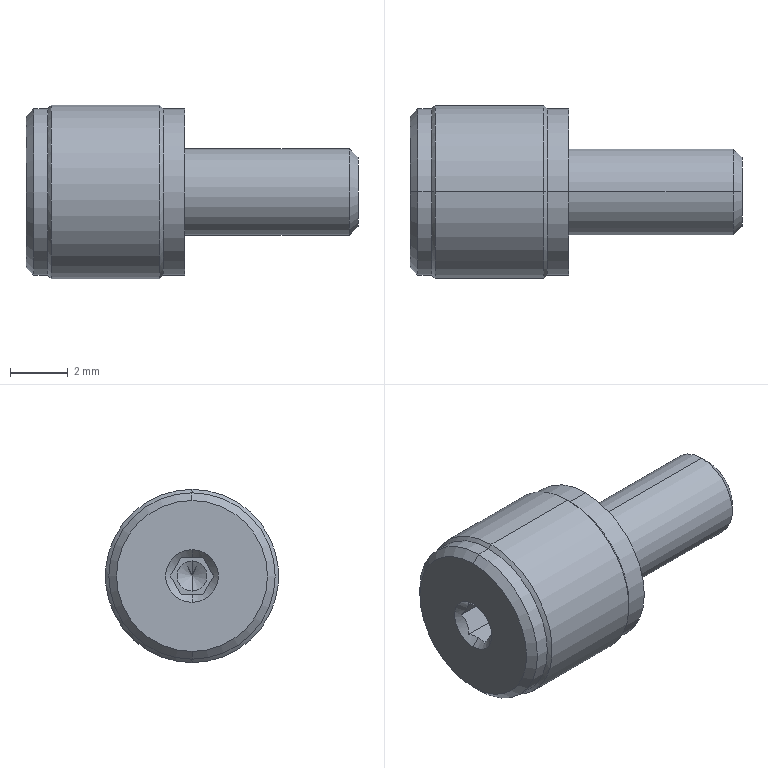Part | SolidWorks | features ICE 1, RevCut 1, Revolution 1 | 1 solid | 32 faces | box 11.5 x 6 x 6 mm | volume 189.881 mm3 | cone 12 | cylinder 10 | plane 10 | commonest cylinder face diameters 5.76 x4 1.04 x2 3 x2 6 x2
STEP:
#1=CARTESIAN_POINT('',(-3.05,0.,-0.52));
#2=VERTEX_POINT('',#1);
#3=CARTESIAN_POINT('',(-3.05,0.,0.52));
#4=VERTEX_POINT('',#3);
#5=CARTESIAN_POINT('',(-3.05,0.,0.));
#6=DIRECTION('',(-1.,0.,0.));
#7=DIRECTION('',(0.,0.,1.));
#8=AXIS2_PLACEMENT_3D('',#5,#6,#7);
#9=CIRCLE('',#8,0.52);
#10=EDGE_CURVE('',#2,#4,#9,.T.);
#11=ORIENTED_EDGE('',*,*,#10,.F.);
#12=CARTESIAN_POINT('',(-3.667,0.,-0.52));
#13=VERTEX_POINT('',#12);
#14=CARTESIAN_POINT('',(-2.75,0.,-0.52));
#15=DIRECTION('',(-1.,0.,0.));
#16=VECTOR('',#15,1000.);
#17=LINE('',#14,#16);
#18=EDGE_CURVE('',#2,#13,#17,.T.);
#19=ORIENTED_EDGE('',*,*,#18,.T.);
#20=CARTESIAN_POINT('',(-3.667,0.,0.52));
#21=VERTEX_POINT('',#20);
#22=CARTESIAN_POINT('',(-3.667,0.,0.));
#23=DIRECTION('',(1.,0.,0.));
#24=DIRECTION('',(0.,0.,-1.));
#25=AXIS2_PLACEMENT_3D('',#22,#23,#24);
#26=CIRCLE('',#25,0.52);
#27=EDGE_CURVE('',#21,#13,#26,.T.);
#28=ORIENTED_EDGE('',*,*,#27,.F.);
#29=CARTESIAN_POINT('',(-2.75,0.,0.52));
#30=DIRECTION('',(-1.,0.,0.));
#31=VECTOR('',#30,1000.);
#32=LINE('',#29,#31);
#33=EDGE_CURVE('',#4,#21,#32,.T.);
#34=ORIENTED_EDGE('',*,*,#33,.F.);
#35=EDGE_LOOP('',(#11,#19,#28,#34));
#36=FACE_OUTER_BOUND('',#35,.T.);
#37=CARTESIAN_POINT('',(-2.75,0.,0.));
#38=DIRECTION('',(-1.,0.,0.));
#39=DIRECTION('',(0.,0.,1.));
#40=AXIS2_PLACEMENT_3D('',#37,#38,#39);
#41=CYLINDRICAL_SURFACE('',#40,0.52);
#42=ADVANCED_FACE('',(#36),#41,.F.);
#43=CARTESIAN_POINT('',(-2.75,0.,0.));
#44=VERTEX_POINT('',#43);
#45=CARTESIAN_POINT('',(-2.75,0.,0.));
#46=DIRECTION('',(-0.5,0.,0.866));
#47=VECTOR('',#46,1000.);
#48=LINE('',#45,#47);
#49=EDGE_CURVE('',#44,#4,#48,.T.);
#50=ORIENTED_EDGE('',*,*,#49,.F.);
#51=CARTESIAN_POINT('',(-2.75,0.,0.));
#52=DIRECTION('',(-0.5,0.,-0.866));
#53=VECTOR('',#52,1000.);
#54=LINE('',#51,#53);
#55=EDGE_CURVE('',#44,#2,#54,.T.);
#56=ORIENTED_EDGE('',*,*,#55,.T.);
#57=ORIENTED_EDGE('',*,*,#10,.T.);
#58=EDGE_LOOP('',(#50,#56,#57));
#59=FACE_OUTER_BOUND('',#58,.T.);
#60=CARTESIAN_POINT('',(-1002.75,0.,0.));
#61=DIRECTION('',(-1.,0.,0.));
#62=DIRECTION('',(0.,0.,1.));
#63=AXIS2_PLACEMENT_3D('',#60,#61,#62);
#64=CONICAL_SURFACE('',#63,1732.051,1.047);
#65=ADVANCED_FACE('',(#59),#64,.F.);
#66=CARTESIAN_POINT('',(6.,0.,1.194));
#67=VERTEX_POINT('',#66);
#68=CARTESIAN_POINT('',(6.,0.,-1.194));
#69=VERTEX_POINT('',#68);
#70=CARTESIAN_POINT('',(6.,0.,0.));
#71=DIRECTION('',(-1.,0.,0.));
#72=DIRECTION('',(0.,0.,1.));
#73=AXIS2_PLACEMENT_3D('',#70,#71,#72);
#74=CIRCLE('',#73,1.194);
#75=EDGE_CURVE('',#67,#69,#74,.T.);
#76=ORIENTED_EDGE('',*,*,#75,.T.);
#77=CARTESIAN_POINT('',(5.694,0.,-1.5));
#78=VERTEX_POINT('',#77);
#79=CARTESIAN_POINT('',(6.,0.,-1.194));
#80=DIRECTION('',(-0.7071,0.,-0.7071));
#81=VECTOR('',#80,1000.);
#82=LINE('',#79,#81);
#83=EDGE_CURVE('',#69,#78,#82,.T.);
#84=ORIENTED_EDGE('',*,*,#83,.T.);
#85=CARTESIAN_POINT('',(5.694,0.,1.5));
#86=VERTEX_POINT('',#85);
#87=CARTESIAN_POINT('',(5.694,0.,0.));
#88=DIRECTION('',(-1.,0.,0.));
#89=DIRECTION('',(0.,0.,1.));
#90=AXIS2_PLACEMENT_3D('',#87,#88,#89);
#91=CIRCLE('',#90,1.5);
#92=EDGE_CURVE('',#86,#78,#91,.T.);
#93=ORIENTED_EDGE('',*,*,#92,.F.);
#94=CARTESIAN_POINT('',(6.,0.,1.194));
#95=DIRECTION('',(-0.7071,0.,0.7071));
#96=VECTOR('',#95,1000.);
#97=LINE('',#94,#96);
#98=EDGE_CURVE('',#67,#86,#97,.T.);
#99=ORIENTED_EDGE('',*,*,#98,.F.);
#100=EDGE_LOOP('',(#76,#84,#93,#99));
#101=FACE_OUTER_BOUND('',#100,.T.);
#102=CARTESIAN_POINT('',(6.,0.,0.));
#103=DIRECTION('',(-1.,0.,0.));
#104=DIRECTION('',(0.,0.,1.));
#105=AXIS2_PLACEMENT_3D('',#102,#103,#104);
#106=CONICAL_SURFACE('',#105,1.194,0.7854);
#107=ADVANCED_FACE('',(#101),#106,.T.);
#108=ORIENTED_EDGE('',*,*,#92,.T.);
#109=CARTESIAN_POINT('',(0.,0.,-1.5));
#110=VERTEX_POINT('',#109);
#111=CARTESIAN_POINT('',(6.,0.,-1.5));
#112=DIRECTION('',(-1.,0.,0.));
#113=VECTOR('',#112,1000.);
#114=LINE('',#111,#113);
#115=EDGE_CURVE('',#78,#110,#114,.T.);
#116=ORIENTED_EDGE('',*,*,#115,.T.);
#117=CARTESIAN_POINT('',(0.,0.,1.5));
#118=VERTEX_POINT('',#117);
#119=CARTESIAN_POINT('',(0.,0.,0.));
#120=DIRECTION('',(-1.,0.,0.));
#121=DIRECTION('',(0.,0.,1.));
#122=AXIS2_PLACEMENT_3D('',#119,#120,#121);
#123=CIRCLE('',#122,1.5);
#124=EDGE_CURVE('',#118,#110,#123,.T.);
#125=ORIENTED_EDGE('',*,*,#124,.F.);
#126=CARTESIAN_POINT('',(6.,0.,1.5));
#127=DIRECTION('',(-1.,0.,0.));
#128=VECTOR('',#127,1000.);
#129=LINE('',#126,#128);
#130=EDGE_CURVE('',#86,#118,#129,.T.);
#131=ORIENTED_EDGE('',*,*,#130,.F.);
#132=EDGE_LOOP('',(#108,#116,#125,#131));
#133=FACE_OUTER_BOUND('',#132,.T.);
#134=CARTESIAN_POINT('',(6.,0.,0.));
#135=DIRECTION('',(-1.,0.,0.));
#136=DIRECTION('',(0.,0.,1.));
#137=AXIS2_PLACEMENT_3D('',#134,#135,#136);
#138=CYLINDRICAL_SURFACE('',#137,1.5);
#139=ADVANCED_FACE('',(#133),#138,.T.);
#140=CARTESIAN_POINT('',(0.,0.,2.88));
#141=VERTEX_POINT('',#140);
#142=CARTESIAN_POINT('',(0.,0.,-2.88));
#143=VERTEX_POINT('',#142);
#144=CARTESIAN_POINT('',(0.,0.,0.));
#145=DIRECTION('',(-1.,0.,0.));
#146=DIRECTION('',(0.,0.,1.));
#147=AXIS2_PLACEMENT_3D('',#144,#145,#146);
#148=CIRCLE('',#147,2.88);
#149=EDGE_CURVE('',#141,#143,#148,.T.);
#150=ORIENTED_EDGE('',*,*,#149,.T.);
#151=CARTESIAN_POINT('',(-0.75,0.,-2.88));
#152=VERTEX_POINT('',#151);
#153=CARTESIAN_POINT('',(6.,0.,-2.88));
#154=DIRECTION('',(-1.,0.,0.));
#155=VECTOR('',#154,1000.);
#156=LINE('',#153,#155);
#157=EDGE_CURVE('',#143,#152,#156,.T.);
#158=ORIENTED_EDGE('',*,*,#157,.T.);
#159=CARTESIAN_POINT('',(-0.75,0.,2.88));
#160=VERTEX_POINT('',#159);
#161=CARTESIAN_POINT('',(-0.75,0.,0.));
#162=DIRECTION('',(-1.,0.,0.));
#163=DIRECTION('',(0.,0.,1.));
#164=AXIS2_PLACEMENT_3D('',#161,#162,#163);
#165=CIRCLE('',#164,2.88);
#166=EDGE_CURVE('',#160,#152,#165,.T.);
#167=ORIENTED_EDGE('',*,*,#166,.F.);
#168=CARTESIAN_POINT('',(6.,0.,2.88));
#169=DIRECTION('',(-1.,0.,0.));
#170=VECTOR('',#169,1000.);
#171=LINE('',#168,#170);
#172=EDGE_CURVE('',#141,#160,#171,.T.);
#173=ORIENTED_EDGE('',*,*,#172,.F.);
#174=EDGE_LOOP('',(#150,#158,#167,#173));
#175=FACE_OUTER_BOUND('',#174,.T.);
#176=CARTESIAN_POINT('',(6.,0.,0.));
#177=DIRECTION('',(-1.,0.,0.));
#178=DIRECTION('',(0.,0.,1.));
#179=AXIS2_PLACEMENT_3D('',#176,#177,#178);
#180=CYLINDRICAL_SURFACE('',#179,2.88);
#181=ADVANCED_FACE('',(#175),#180,.T.);
#182=ORIENTED_EDGE('',*,*,#166,.T.);
#183=CARTESIAN_POINT('',(-0.87,0.,-3.));
#184=VERTEX_POINT('',#183);
#185=CARTESIAN_POINT('',(-0.75,0.,-2.88));
#186=DIRECTION('',(-0.7071,0.,-0.7071));
#187=VECTOR('',#186,1000.);
#188=LINE('',#185,#187);
#189=EDGE_CURVE('',#152,#184,#188,.T.);
#190=ORIENTED_EDGE('',*,*,#189,.T.);
#191=CARTESIAN_POINT('',(-0.87,0.,3.));
#192=VERTEX_POINT('',#191);
#193=CARTESIAN_POINT('',(-0.87,0.,0.));
#194=DIRECTION('',(-1.,0.,0.));
#195=DIRECTION('',(0.,0.,1.));
#196=AXIS2_PLACEMENT_3D('',#193,#194,#195);
#197=CIRCLE('',#196,3.);
#198=EDGE_CURVE('',#192,#184,#197,.T.);
#199=ORIENTED_EDGE('',*,*,#198,.F.);
#200=CARTESIAN_POINT('',(-0.75,0.,2.88));
#201=DIRECTION('',(-0.7071,0.,0.7071));
#202=VECTOR('',#201,1000.);
#203=LINE('',#200,#202);
#204=EDGE_CURVE('',#160,#192,#203,.T.);
#205=ORIENTED_EDGE('',*,*,#204,.F.);
#206=EDGE_LOOP('',(#182,#190,#199,#205));
#207=FACE_OUTER_BOUND('',#206,.T.);
#208=CARTESIAN_POINT('',(-0.75,0.,0.));
#209=DIRECTION('',(-1.,0.,0.));
#210=DIRECTION('',(0.,0.,1.));
#211=AXIS2_PLACEMENT_3D('',#208,#209,#210);
#212=CONICAL_SURFACE('',#211,2.88,0.7854);
#213=ADVANCED_FACE('',(#207),#212,.T.);
#214=ORIENTED_EDGE('',*,*,#198,.T.);
#215=CARTESIAN_POINT('',(-4.63,0.,-3.));
#216=VERTEX_POINT('',#215);
#217=CARTESIAN_POINT('',(6.,0.,-3.));
#218=DIRECTION('',(-1.,0.,0.));
#219=VECTOR('',#218,1000.);
#220=LINE('',#217,#219);
#221=EDGE_CURVE('',#184,#216,#220,.T.);
#222=ORIENTED_EDGE('',*,*,#221,.T.);
#223=CARTESIAN_POINT('',(-4.63,0.,3.));
#224=VERTEX_POINT('',#223);
#225=CARTESIAN_POINT('',(-4.63,0.,0.));
#226=DIRECTION('',(-1.,0.,0.));
#227=DIRECTION('',(0.,0.,1.));
#228=AXIS2_PLACEMENT_3D('',#225,#226,#227);
#229=CIRCLE('',#228,3.);
#230=EDGE_CURVE('',#224,#216,#229,.T.);
#231=ORIENTED_EDGE('',*,*,#230,.F.);
#232=CARTESIAN_POINT('',(6.,0.,3.));
#233=DIRECTION('',(-1.,0.,0.));
#234=VECTOR('',#233,1000.);
#235=LINE('',#232,#234);
#236=EDGE_CURVE('',#192,#224,#235,.T.);
#237=ORIENTED_EDGE('',*,*,#236,.F.);
#238=EDGE_LOOP('',(#214,#222,#231,#237));
#239=FACE_OUTER_BOUND('',#238,.T.);
#240=CARTESIAN_POINT('',(6.,0.,0.));
#241=DIRECTION('',(-1.,0.,0.));
#242=DIRECTION('',(0.,0.,1.));
#243=AXIS2_PLACEMENT_3D('',#240,#241,#242);
#244=CYLINDRICAL_SURFACE('',#243,3.);
#245=ADVANCED_FACE('',(#239),#244,.T.);
#246=CARTESIAN_POINT('',(-4.75,0.,2.88));
#247=VERTEX_POINT('',#246);
#248=CARTESIAN_POINT('',(-4.75,0.,-2.88));
#249=VERTEX_POINT('',#248);
#250=CARTESIAN_POINT('',(-4.75,0.,0.));
#251=DIRECTION('',(-1.,0.,0.));
#252=DIRECTION('',(0.,0.,1.));
#253=AXIS2_PLACEMENT_3D('',#250,#251,#252);
#254=CIRCLE('',#253,2.88);
#255=EDGE_CURVE('',#247,#249,#254,.T.);
#256=ORIENTED_EDGE('',*,*,#255,.F.);
#257=CARTESIAN_POINT('',(-4.63,0.,3.));
#258=DIRECTION('',(0.7071,0.,0.7071));
#259=VECTOR('',#258,1000.);
#260=LINE('',#257,#259);
#261=EDGE_CURVE('',#247,#224,#260,.T.);
#262=ORIENTED_EDGE('',*,*,#261,.T.);
#263=ORIENTED_EDGE('',*,*,#230,.T.);
#264=CARTESIAN_POINT('',(-4.63,0.,-3.));
#265=DIRECTION('',(0.7071,0.,-0.7071));
#266=VECTOR('',#265,1000.);
#267=LINE('',#264,#266);
#268=EDGE_CURVE('',#249,#216,#267,.T.);
#269=ORIENTED_EDGE('',*,*,#268,.F.);
#270=EDGE_LOOP('',(#256,#262,#263,#269));
#271=FACE_OUTER_BOUND('',#270,.T.);
#272=CARTESIAN_POINT('',(-4.63,0.,0.));
#273=DIRECTION('',(1.,0.,0.));
#274=DIRECTION('',(0.,0.,-1.));
#275=AXIS2_PLACEMENT_3D('',#272,#273,#274);
#276=CONICAL_SURFACE('',#275,3.,0.7854);
#277=ADVANCED_FACE('',(#271),#276,.T.);
#278=ORIENTED_EDGE('',*,*,#255,.T.);
#279=CARTESIAN_POINT('',(-5.235,0.,-2.88));
#280=VERTEX_POINT('',#279);
#281=CARTESIAN_POINT('',(6.,0.,-2.88));
#282=DIRECTION('',(-1.,0.,0.));
#283=VECTOR('',#282,1000.);
#284=LINE('',#281,#283);
#285=EDGE_CURVE('',#249,#280,#284,.T.);
#286=ORIENTED_EDGE('',*,*,#285,.T.);
#287=CARTESIAN_POINT('',(-5.235,0.,2.88));
#288=VERTEX_POINT('',#287);
#289=CARTESIAN_POINT('',(-5.235,0.,0.));
#290=DIRECTION('',(-1.,0.,0.));
#291=DIRECTION('',(0.,0.,1.));
#292=AXIS2_PLACEMENT_3D('',#289,#290,#291);
#293=CIRCLE('',#292,2.88);
#294=EDGE_CURVE('',#288,#280,#293,.T.);
#295=ORIENTED_EDGE('',*,*,#294,.F.);
#296=CARTESIAN_POINT('',(6.,0.,2.88));
#297=DIRECTION('',(-1.,0.,0.));
#298=VECTOR('',#297,1000.);
#299=LINE('',#296,#298);
#300=EDGE_CURVE('',#247,#288,#299,.T.);
#301=ORIENTED_EDGE('',*,*,#300,.F.);
#302=EDGE_LOOP('',(#278,#286,#295,#301));
#303=FACE_OUTER_BOUND('',#302,.T.);
#304=CARTESIAN_POINT('',(6.,0.,0.));
#305=DIRECTION('',(-1.,0.,0.));
#306=DIRECTION('',(0.,0.,1.));
#307=AXIS2_PLACEMENT_3D('',#304,#305,#306);
#308=CYLINDRICAL_SURFACE('',#307,2.88);
#309=ADVANCED_FACE('',(#303),#308,.T.);
#310=CARTESIAN_POINT('',(-5.5,0.,2.615));
#311=VERTEX_POINT('',#310);
#312=CARTESIAN_POINT('',(-5.5,0.,-2.615));
#313=VERTEX_POINT('',#312);
#314=CARTESIAN_POINT('',(-5.5,0.,0.));
#315=DIRECTION('',(-1.,0.,0.));
#316=DIRECTION('',(0.,0.,1.));
#317=AXIS2_PLACEMENT_3D('',#314,#315,#316);
#318=CIRCLE('',#317,2.615);
#319=EDGE_CURVE('',#311,#313,#318,.T.);
#320=ORIENTED_EDGE('',*,*,#319,.F.);
#321=CARTESIAN_POINT('',(-5.235,0.,2.88));
#322=DIRECTION('',(0.7071,0.,0.7071));
#323=VECTOR('',#322,1000.);
#324=LINE('',#321,#323);
#325=EDGE_CURVE('',#311,#288,#324,.T.);
#326=ORIENTED_EDGE('',*,*,#325,.T.);
#327=ORIENTED_EDGE('',*,*,#294,.T.);
#328=CARTESIAN_POINT('',(-5.235,0.,-2.88));
#329=DIRECTION('',(0.7071,0.,-0.7071));
#330=VECTOR('',#329,1000.);
#331=LINE('',#328,#330);
#332=EDGE_CURVE('',#313,#280,#331,.T.);
#333=ORIENTED_EDGE('',*,*,#332,.F.);
#334=EDGE_LOOP('',(#320,#326,#327,#333));
#335=FACE_OUTER_BOUND('',#334,.T.);
#336=CARTESIAN_POINT('',(-5.235,0.,0.));
#337=DIRECTION('',(1.,0.,0.));
#338=DIRECTION('',(0.,0.,-1.));
#339=AXIS2_PLACEMENT_3D('',#336,#337,#338);
#340=CONICAL_SURFACE('',#339,2.88,0.7854);
#341=ADVANCED_FACE('',(#335),#340,.T.);
#342=CARTESIAN_POINT('',(-5.341,-0.3753,-0.65));
#343=VERTEX_POINT('',#342);
#344=CARTESIAN_POINT('',(-5.24,0.,-0.65));
#345=VERTEX_POINT('',#344);
#346=CARTESIAN_POINT('',(-5.341,-0.3753,-0.65));
#347=CARTESIAN_POINT('',(-5.282,-0.2585,-0.65));
#348=CARTESIAN_POINT('',(-5.24,-0.1313,-0.65));
#349=CARTESIAN_POINT('',(-5.24,0.,-0.65));
#350=B_SPLINE_CURVE_WITH_KNOTS('',3,(#346,#347,#348,#349),.UNSPECIFIED.,.F.,.F.,(4,4),(0.0006064,0.0009955),.UNSPECIFIED.);
#351=EDGE_CURVE('',#343,#345,#350,.T.);
#352=ORIENTED_EDGE('',*,*,#351,.T.);
#353=CARTESIAN_POINT('',(-5.5,0.,-0.91));
#354=VERTEX_POINT('',#353);
#355=CARTESIAN_POINT('',(-5.11,0.,-0.52));
#356=DIRECTION('',(-0.7071,0.,-0.7071));
#357=VECTOR('',#356,1000.);
#358=LINE('',#355,#357);
#359=EDGE_CURVE('',#345,#354,#358,.T.);
#360=ORIENTED_EDGE('',*,*,#359,.T.);
#361=CARTESIAN_POINT('',(-5.5,0.,0.91));
#362=VERTEX_POINT('',#361);
#363=CARTESIAN_POINT('',(-5.5,0.,0.));
#364=DIRECTION('',(-1.,0.,0.));
#365=DIRECTION('',(0.,0.,1.));
#366=AXIS2_PLACEMENT_3D('',#363,#364,#365);
#367=CIRCLE('',#366,0.91);
#368=EDGE_CURVE('',#354,#362,#367,.T.);
#369=ORIENTED_EDGE('',*,*,#368,.T.);
#370=CARTESIAN_POINT('',(-5.24,0.,0.65));
#371=VERTEX_POINT('',#370);
#372=CARTESIAN_POINT('',(-5.11,0.,0.52));
#373=DIRECTION('',(-0.7071,0.,0.7071));
#374=VECTOR('',#373,1000.);
#375=LINE('',#372,#374);
#376=EDGE_CURVE('',#371,#362,#375,.T.);
#377=ORIENTED_EDGE('',*,*,#376,.F.);
#378=CARTESIAN_POINT('',(-5.341,-0.3753,0.65));
#379=VERTEX_POINT('',#378);
#380=CARTESIAN_POINT('',(-5.24,0.,0.65));
#381=CARTESIAN_POINT('',(-5.24,-0.1313,0.65));
#382=CARTESIAN_POINT('',(-5.282,-0.2585,0.65));
#383=CARTESIAN_POINT('',(-5.341,-0.3753,0.65));
#384=B_SPLINE_CURVE_WITH_KNOTS('',3,(#380,#381,#382,#383),.UNSPECIFIED.,.F.,.F.,(4,4),(0.000782,0.001171),.UNSPECIFIED.);
#385=EDGE_CURVE('',#371,#379,#384,.T.);
#386=ORIENTED_EDGE('',*,*,#385,.T.);
#387=CARTESIAN_POINT('',(-5.341,-0.7506,0.));
#388=VERTEX_POINT('',#387);
#389=CARTESIAN_POINT('',(-5.341,-0.3753,0.65));
#390=CARTESIAN_POINT('',(-5.311,-0.4046,0.5992));
#391=CARTESIAN_POINT('',(-5.286,-0.4346,0.5473));
#392=CARTESIAN_POINT('',(-5.251,-0.4967,0.4397));
#393=CARTESIAN_POINT('',(-5.24,-0.5295,0.3829));
#394=CARTESIAN_POINT('',(-5.24,-0.6277,0.2127));
#395=CARTESIAN_POINT('',(-5.282,-0.6916,0.1022));
#396=CARTESIAN_POINT('',(-5.341,-0.7506,0.));
#397=B_SPLINE_CURVE_WITH_KNOTS('',3,(#389,#390,#391,#392,#393,#394,#395,#396),.UNSPECIFIED.,.F.,.F.,(4,2,2,4),(0.000000254,0.0001941,0.0003879,0.0007755),.UNSPECIFIED.);
#398=EDGE_CURVE('',#379,#388,#397,.T.);
#399=ORIENTED_EDGE('',*,*,#398,.T.);
#400=CARTESIAN_POINT('',(-5.341,-0.7506,0.));
#401=CARTESIAN_POINT('',(-5.311,-0.7212,-0.05078));
#402=CARTESIAN_POINT('',(-5.286,-0.6913,-0.1027));
#403=CARTESIAN_POINT('',(-5.251,-0.6291,-0.2103));
#404=CARTESIAN_POINT('',(-5.24,-0.5964,-0.2671));
#405=CARTESIAN_POINT('',(-5.24,-0.4981,-0.4373));
#406=CARTESIAN_POINT('',(-5.282,-0.4343,-0.5478));
#407=CARTESIAN_POINT('',(-5.341,-0.3753,-0.65));
#408=B_SPLINE_CURVE_WITH_KNOTS('',3,(#400,#401,#402,#403,#404,#405,#406,#407),.UNSPECIFIED.,.F.,.F.,(4,2,2,4),(0.000000254,0.0001941,0.0003879,0.0007755),.UNSPECIFIED.);
#409=EDGE_CURVE('',#388,#343,#408,.T.);
#410=ORIENTED_EDGE('',*,*,#409,.T.);
#411=EDGE_LOOP('',(#352,#360,#369,#377,#386,#399,#410));
#412=FACE_OUTER_BOUND('',#411,.T.);
#413=CARTESIAN_POINT('',(-5.11,0.,0.));
#414=DIRECTION('',(-1.,0.,0.));
#415=DIRECTION('',(0.,0.,1.));
#416=AXIS2_PLACEMENT_3D('',#413,#414,#415);
#417=CONICAL_SURFACE('',#416,0.52,0.7854);
#418=ADVANCED_FACE('',(#412),#417,.F.);
#419=ORIENTED_EDGE('',*,*,#359,.F.);
#420=CARTESIAN_POINT('',(-5.341,0.3753,-0.65));
#421=VERTEX_POINT('',#420);
#422=CARTESIAN_POINT('',(-5.24,0.,-0.65));
#423=CARTESIAN_POINT('',(-5.24,0.1316,-0.65));
#424=CARTESIAN_POINT('',(-5.282,0.259,-0.65));
#425=CARTESIAN_POINT('',(-5.341,0.3753,-0.65));
#426=B_SPLINE_CURVE_WITH_KNOTS('',3,(#422,#423,#424,#425),.UNSPECIFIED.,.F.,.F.,(4,4),(0.0009955,0.001385),.UNSPECIFIED.);
#427=EDGE_CURVE('',#345,#421,#426,.T.);
#428=ORIENTED_EDGE('',*,*,#427,.T.);
#429=CARTESIAN_POINT('',(-5.341,0.7506,0.));
#430=VERTEX_POINT('',#429);
#431=CARTESIAN_POINT('',(-5.341,0.3753,-0.65));
#432=CARTESIAN_POINT('',(-5.311,0.4046,-0.5992));
#433=CARTESIAN_POINT('',(-5.286,0.4346,-0.5473));
#434=CARTESIAN_POINT('',(-5.251,0.4967,-0.4397));
#435=CARTESIAN_POINT('',(-5.24,0.5295,-0.3829));
#436=CARTESIAN_POINT('',(-5.24,0.6277,-0.2127));
#437=CARTESIAN_POINT('',(-5.282,0.6916,-0.1022));
#438=CARTESIAN_POINT('',(-5.341,0.7506,0.));
#439=B_SPLINE_CURVE_WITH_KNOTS('',3,(#431,#432,#433,#434,#435,#436,#437,#438),.UNSPECIFIED.,.F.,.F.,(4,2,2,4),(0.000000254,0.0001941,0.0003879,0.0007755),.UNSPECIFIED.);
#440=EDGE_CURVE('',#421,#430,#439,.T.);
#441=ORIENTED_EDGE('',*,*,#440,.T.);
#442=CARTESIAN_POINT('',(-5.341,0.3753,0.65));
#443=VERTEX_POINT('',#442);
#444=CARTESIAN_POINT('',(-5.341,0.7506,0.));
#445=CARTESIAN_POINT('',(-5.311,0.7212,0.05078));
#446=CARTESIAN_POINT('',(-5.286,0.6913,0.1027));
#447=CARTESIAN_POINT('',(-5.251,0.6291,0.2103));
#448=CARTESIAN_POINT('',(-5.24,0.5964,0.2671));
#449=CARTESIAN_POINT('',(-5.24,0.4981,0.4373));
#450=CARTESIAN_POINT('',(-5.282,0.4343,0.5478));
#451=CARTESIAN_POINT('',(-5.341,0.3753,0.65));
#452=B_SPLINE_CURVE_WITH_KNOTS('',3,(#444,#445,#446,#447,#448,#449,#450,#451),.UNSPECIFIED.,.F.,.F.,(4,2,2,4),(0.000000254,0.0001941,0.0003879,0.0007755),.UNSPECIFIED.);
#453=EDGE_CURVE('',#430,#443,#452,.T.);
#454=ORIENTED_EDGE('',*,*,#453,.T.);
#455=CARTESIAN_POINT('',(-5.341,0.3753,0.65));
#456=CARTESIAN_POINT('',(-5.282,0.259,0.65));
#457=CARTESIAN_POINT('',(-5.24,0.1316,0.65));
#458=CARTESIAN_POINT('',(-5.24,0.,0.65));
#459=B_SPLINE_CURVE_WITH_KNOTS('',3,(#455,#456,#457,#458),.UNSPECIFIED.,.F.,.F.,(4,4),(0.0003925,0.000782),.UNSPECIFIED.);
#460=EDGE_CURVE('',#443,#371,#459,.T.);
#461=ORIENTED_EDGE('',*,*,#460,.T.);
#462=ORIENTED_EDGE('',*,*,#376,.T.);
#463=CARTESIAN_POINT('',(-5.5,0.,0.));
#464=DIRECTION('',(-1.,0.,0.));
#465=DIRECTION('',(0.,0.,1.));
#466=AXIS2_PLACEMENT_3D('',#463,#464,#465);
#467=CIRCLE('',#466,0.91);
#468=EDGE_CURVE('',#362,#354,#467,.T.);
#469=ORIENTED_EDGE('',*,*,#468,.T.);
#470=EDGE_LOOP('',(#419,#428,#441,#454,#461,#462,#469));
#471=FACE_OUTER_BOUND('',#470,.T.);
#472=CARTESIAN_POINT('',(-5.11,0.,0.));
#473=DIRECTION('',(-1.,0.,0.));
#474=DIRECTION('',(0.,0.,1.));
#475=AXIS2_PLACEMENT_3D('',#472,#473,#474);
#476=CONICAL_SURFACE('',#475,0.52,0.7854);
#477=ADVANCED_FACE('',(#471),#476,.F.);
#478=CARTESIAN_POINT('',(-5.5,0.,0.));
#479=DIRECTION('',(-1.,0.,0.));
#480=DIRECTION('',(0.,0.,1.));
#481=AXIS2_PLACEMENT_3D('',#478,#479,#480);
#482=CIRCLE('',#481,2.615);
#483=EDGE_CURVE('',#313,#311,#482,.T.);
#484=ORIENTED_EDGE('',*,*,#483,.T.);
#485=ORIENTED_EDGE('',*,*,#319,.T.);
#486=EDGE_LOOP('',(#484,#485));
#487=FACE_OUTER_BOUND('',#486,.T.);
#488=ORIENTED_EDGE('',*,*,#468,.F.);
#489=ORIENTED_EDGE('',*,*,#368,.F.);
#490=EDGE_LOOP('',(#488,#489));
#491=FACE_BOUND('',#490,.T.);
#492=CARTESIAN_POINT('',(-5.5,0.,0.));
#493=DIRECTION('',(1.,0.,0.));
#494=DIRECTION('',(0.,0.,-1.));
#495=AXIS2_PLACEMENT_3D('',#492,#493,#494);
#496=PLANE('',#495);
#497=ADVANCED_FACE('',(#487,#491),#496,.F.);
#498=ORIENTED_EDGE('',*,*,#325,.F.);
#499=ORIENTED_EDGE('',*,*,#483,.F.);
#500=ORIENTED_EDGE('',*,*,#332,.T.);
#501=CARTESIAN_POINT('',(-5.235,0.,0.));
#502=DIRECTION('',(-1.,0.,0.));
#503=DIRECTION('',(0.,0.,1.));
#504=AXIS2_PLACEMENT_3D('',#501,#502,#503);
#505=CIRCLE('',#504,2.88);
#506=EDGE_CURVE('',#280,#288,#505,.T.);
#507=ORIENTED_EDGE('',*,*,#506,.T.);
#508=EDGE_LOOP('',(#498,#499,#500,#507));
#509=FACE_OUTER_BOUND('',#508,.T.);
#510=CARTESIAN_POINT('',(-5.235,0.,0.));
#511=DIRECTION('',(1.,0.,0.));
#512=DIRECTION('',(0.,0.,-1.));
#513=AXIS2_PLACEMENT_3D('',#510,#511,#512);
#514=CONICAL_SURFACE('',#513,2.88,0.7854);
#515=ADVANCED_FACE('',(#509),#514,.T.);
#516=ORIENTED_EDGE('',*,*,#285,.F.);
#517=CARTESIAN_POINT('',(-4.75,0.,0.));
#518=DIRECTION('',(-1.,0.,0.));
#519=DIRECTION('',(0.,0.,1.));
#520=AXIS2_PLACEMENT_3D('',#517,#518,#519);
#521=CIRCLE('',#520,2.88);
#522=EDGE_CURVE('',#249,#247,#521,.T.);
#523=ORIENTED_EDGE('',*,*,#522,.T.);
#524=ORIENTED_EDGE('',*,*,#300,.T.);
#525=ORIENTED_EDGE('',*,*,#506,.F.);
#526=EDGE_LOOP('',(#516,#523,#524,#525));
#527=FACE_OUTER_BOUND('',#526,.T.);
#528=CARTESIAN_POINT('',(6.,0.,0.));
#529=DIRECTION('',(-1.,0.,0.));
#530=DIRECTION('',(0.,0.,1.));
#531=AXIS2_PLACEMENT_3D('',#528,#529,#530);
#532=CYLINDRICAL_SURFACE('',#531,2.88);
#533=ADVANCED_FACE('',(#527),#532,.T.);
#534=ORIENTED_EDGE('',*,*,#261,.F.);
#535=ORIENTED_EDGE('',*,*,#522,.F.);
#536=ORIENTED_EDGE('',*,*,#268,.T.);
#537=CARTESIAN_POINT('',(-4.63,0.,0.));
#538=DIRECTION('',(-1.,0.,0.));
#539=DIRECTION('',(0.,0.,1.));
#540=AXIS2_PLACEMENT_3D('',#537,#538,#539);
#541=CIRCLE('',#540,3.);
#542=EDGE_CURVE('',#216,#224,#541,.T.);
#543=ORIENTED_EDGE('',*,*,#542,.T.);
#544=EDGE_LOOP('',(#534,#535,#536,#543));
#545=FACE_OUTER_BOUND('',#544,.T.);
#546=CARTESIAN_POINT('',(-4.63,0.,0.));
#547=DIRECTION('',(1.,0.,0.));
#548=DIRECTION('',(0.,0.,-1.));
#549=AXIS2_PLACEMENT_3D('',#546,#547,#548);
#550=CONICAL_SURFACE('',#549,3.,0.7854);
#551=ADVANCED_FACE('',(#545),#550,.T.);
#552=ORIENTED_EDGE('',*,*,#221,.F.);
#553=CARTESIAN_POINT('',(-0.87,0.,0.));
#554=DIRECTION('',(-1.,0.,0.));
#555=DIRECTION('',(0.,0.,1.));
#556=AXIS2_PLACEMENT_3D('',#553,#554,#555);
#557=CIRCLE('',#556,3.);
#558=EDGE_CURVE('',#184,#192,#557,.T.);
#559=ORIENTED_EDGE('',*,*,#558,.T.);
#560=ORIENTED_EDGE('',*,*,#236,.T.);
#561=ORIENTED_EDGE('',*,*,#542,.F.);
#562=EDGE_LOOP('',(#552,#559,#560,#561));
#563=FACE_OUTER_BOUND('',#562,.T.);
#564=CARTESIAN_POINT('',(6.,0.,0.));
#565=DIRECTION('',(-1.,0.,0.));
#566=DIRECTION('',(0.,0.,1.));
#567=AXIS2_PLACEMENT_3D('',#564,#565,#566);
#568=CYLINDRICAL_SURFACE('',#567,3.);
#569=ADVANCED_FACE('',(#563),#568,.T.);
#570=ORIENTED_EDGE('',*,*,#189,.F.);
#571=CARTESIAN_POINT('',(-0.75,0.,0.));
#572=DIRECTION('',(-1.,0.,0.));
#573=DIRECTION('',(0.,0.,1.));
#574=AXIS2_PLACEMENT_3D('',#571,#572,#573);
#575=CIRCLE('',#574,2.88);
#576=EDGE_CURVE('',#152,#160,#575,.T.);
#577=ORIENTED_EDGE('',*,*,#576,.T.);
#578=ORIENTED_EDGE('',*,*,#204,.T.);
#579=ORIENTED_EDGE('',*,*,#558,.F.);
#580=EDGE_LOOP('',(#570,#577,#578,#579));
#581=FACE_OUTER_BOUND('',#580,.T.);
#582=CARTESIAN_POINT('',(-0.75,0.,0.));
#583=DIRECTION('',(-1.,0.,0.));
#584=DIRECTION('',(0.,0.,1.));
#585=AXIS2_PLACEMENT_3D('',#582,#583,#584);
#586=CONICAL_SURFACE('',#585,2.88,0.7854);
#587=ADVANCED_FACE('',(#581),#586,.T.);
#588=ORIENTED_EDGE('',*,*,#157,.F.);
#589=CARTESIAN_POINT('',(0.,0.,0.));
#590=DIRECTION('',(-1.,0.,0.));
#591=DIRECTION('',(0.,0.,1.));
#592=AXIS2_PLACEMENT_3D('',#589,#590,#591);
#593=CIRCLE('',#592,2.88);
#594=EDGE_CURVE('',#143,#141,#593,.T.);
#595=ORIENTED_EDGE('',*,*,#594,.T.);
#596=ORIENTED_EDGE('',*,*,#172,.T.);
#597=ORIENTED_EDGE('',*,*,#576,.F.);
#598=EDGE_LOOP('',(#588,#595,#596,#597));
#599=FACE_OUTER_BOUND('',#598,.T.);
#600=CARTESIAN_POINT('',(6.,0.,0.));
#601=DIRECTION('',(-1.,0.,0.));
#602=DIRECTION('',(0.,0.,1.));
#603=AXIS2_PLACEMENT_3D('',#600,#601,#602);
#604=CYLINDRICAL_SURFACE('',#603,2.88);
#605=ADVANCED_FACE('',(#599),#604,.T.);
#606=ORIENTED_EDGE('',*,*,#149,.F.);
#607=ORIENTED_EDGE('',*,*,#594,.F.);
#608=EDGE_LOOP('',(#606,#607));
#609=FACE_OUTER_BOUND('',#608,.T.);
#610=ORIENTED_EDGE('',*,*,#124,.T.);
#611=CARTESIAN_POINT('',(0.,0.,0.));
#612=DIRECTION('',(-1.,0.,0.));
#613=DIRECTION('',(0.,0.,1.));
#614=AXIS2_PLACEMENT_3D('',#611,#612,#613);
#615=CIRCLE('',#614,1.5);
#616=EDGE_CURVE('',#110,#118,#615,.T.);
#617=ORIENTED_EDGE('',*,*,#616,.T.);
#618=EDGE_LOOP('',(#610,#617));
#619=FACE_BOUND('',#618,.T.);
#620=CARTESIAN_POINT('',(0.,2.88,0.));
#621=DIRECTION('',(-1.,0.,0.));
#622=DIRECTION('',(0.,0.,1.));
#623=AXIS2_PLACEMENT_3D('',#620,#621,#622);
#624=PLANE('',#623);
#625=ADVANCED_FACE('',(#609,#619),#624,.F.);
#626=ORIENTED_EDGE('',*,*,#115,.F.);
#627=CARTESIAN_POINT('',(5.694,0.,0.));
#628=DIRECTION('',(-1.,0.,0.));
#629=DIRECTION('',(0.,0.,1.));
#630=AXIS2_PLACEMENT_3D('',#627,#628,#629);
#631=CIRCLE('',#630,1.5);
#632=EDGE_CURVE('',#78,#86,#631,.T.);
#633=ORIENTED_EDGE('',*,*,#632,.T.);
#634=ORIENTED_EDGE('',*,*,#130,.T.);
#635=ORIENTED_EDGE('',*,*,#616,.F.);
#636=EDGE_LOOP('',(#626,#633,#634,#635));
#637=FACE_OUTER_BOUND('',#636,.T.);
#638=CARTESIAN_POINT('',(6.,0.,0.));
#639=DIRECTION('',(-1.,0.,0.));
#640=DIRECTION('',(0.,0.,1.));
#641=AXIS2_PLACEMENT_3D('',#638,#639,#640);
#642=CYLINDRICAL_SURFACE('',#641,1.5);
#643=ADVANCED_FACE('',(#637),#642,.T.);
#644=ORIENTED_EDGE('',*,*,#83,.F.);
#645=CARTESIAN_POINT('',(6.,0.,0.));
#646=DIRECTION('',(-1.,0.,0.));
#647=DIRECTION('',(0.,0.,1.));
#648=AXIS2_PLACEMENT_3D('',#645,#646,#647);
#649=CIRCLE('',#648,1.194);
#650=EDGE_CURVE('',#69,#67,#649,.T.);
#651=ORIENTED_EDGE('',*,*,#650,.T.);
#652=ORIENTED_EDGE('',*,*,#98,.T.);
#653=ORIENTED_EDGE('',*,*,#632,.F.);
#654=EDGE_LOOP('',(#644,#651,#652,#653));
#655=FACE_OUTER_BOUND('',#654,.T.);
#656=CARTESIAN_POINT('',(6.,0.,0.));
#657=DIRECTION('',(-1.,0.,0.));
#658=DIRECTION('',(0.,0.,1.));
#659=AXIS2_PLACEMENT_3D('',#656,#657,#658);
#660=CONICAL_SURFACE('',#659,1.194,0.7854);
#661=ADVANCED_FACE('',(#655),#660,.T.);
#662=ORIENTED_EDGE('',*,*,#75,.F.);
#663=ORIENTED_EDGE('',*,*,#650,.F.);
#664=EDGE_LOOP('',(#662,#663));
#665=FACE_OUTER_BOUND('',#664,.T.);
#666=CARTESIAN_POINT('',(6.,1.194,0.));
#667=DIRECTION('',(-1.,0.,0.));
#668=DIRECTION('',(0.,0.,1.));
#669=AXIS2_PLACEMENT_3D('',#666,#667,#668);
#670=PLANE('',#669);
#671=ADVANCED_FACE('',(#665),#670,.F.);
#672=CARTESIAN_POINT('',(-3.667,0.7506,0.));
#673=VERTEX_POINT('',#672);
#674=CARTESIAN_POINT('',(-3.667,0.7506,0.));
#675=DIRECTION('',(-1.,0.,0.));
#676=VECTOR('',#675,1000.);
#677=LINE('',#674,#676);
#678=EDGE_CURVE('',#673,#430,#677,.T.);
#679=ORIENTED_EDGE('',*,*,#678,.F.);
#680=CARTESIAN_POINT('',(-3.667,0.3753,0.65));
#681=VERTEX_POINT('',#680);
#682=CARTESIAN_POINT('',(-3.667,0.7506,0.));
#683=DIRECTION('',(0.,-0.5,0.866));
#684=VECTOR('',#683,1000.);
#685=LINE('',#682,#684);
#686=EDGE_CURVE('',#673,#681,#685,.T.);
#687=ORIENTED_EDGE('',*,*,#686,.T.);
#688=CARTESIAN_POINT('',(-3.667,0.3753,0.65));
#689=DIRECTION('',(-1.,0.,0.));
#690=VECTOR('',#689,1000.);
#691=LINE('',#688,#690);
#692=EDGE_CURVE('',#681,#443,#691,.T.);
#693=ORIENTED_EDGE('',*,*,#692,.T.);
#694=ORIENTED_EDGE('',*,*,#453,.F.);
#695=EDGE_LOOP('',(#679,#687,#693,#694));
#696=FACE_OUTER_BOUND('',#695,.T.);
#697=CARTESIAN_POINT('',(-3.667,0.7506,0.));
#698=DIRECTION('',(0.,-0.866,-0.5));
#699=DIRECTION('',(0.,0.5,-0.866));
#700=AXIS2_PLACEMENT_3D('',#697,#698,#699);
#701=PLANE('',#700);
#702=ADVANCED_FACE('',(#696),#701,.T.);
#703=ORIENTED_EDGE('',*,*,#692,.F.);
#704=CARTESIAN_POINT('',(-3.667,-0.3753,0.65));
#705=VERTEX_POINT('',#704);
#706=CARTESIAN_POINT('',(-3.667,0.3753,0.65));
#707=DIRECTION('',(0.,-1.,0.));
#708=VECTOR('',#707,1000.);
#709=LINE('',#706,#708);
#710=EDGE_CURVE('',#681,#705,#709,.T.);
#711=ORIENTED_EDGE('',*,*,#710,.T.);
#712=CARTESIAN_POINT('',(-3.667,-0.3753,0.65));
#713=DIRECTION('',(-1.,0.,0.));
#714=VECTOR('',#713,1000.);
#715=LINE('',#712,#714);
#716=EDGE_CURVE('',#705,#379,#715,.T.);
#717=ORIENTED_EDGE('',*,*,#716,.T.);
#718=ORIENTED_EDGE('',*,*,#385,.F.);
#719=ORIENTED_EDGE('',*,*,#460,.F.);
#720=EDGE_LOOP('',(#703,#711,#717,#718,#719));
#721=FACE_OUTER_BOUND('',#720,.T.);
#722=CARTESIAN_POINT('',(-3.667,0.3753,0.65));
#723=DIRECTION('',(0.,0.,-1.));
#724=DIRECTION('',(-1.,0.,0.));
#725=AXIS2_PLACEMENT_3D('',#722,#723,#724);
#726=PLANE('',#725);
#727=ADVANCED_FACE('',(#721),#726,.T.);
#728=ORIENTED_EDGE('',*,*,#716,.F.);
#729=CARTESIAN_POINT('',(-3.667,-0.7506,0.));
#730=VERTEX_POINT('',#729);
#731=CARTESIAN_POINT('',(-3.667,-0.3753,0.65));
#732=DIRECTION('',(0.,-0.5,-0.866));
#733=VECTOR('',#732,1000.);
#734=LINE('',#731,#733);
#735=EDGE_CURVE('',#705,#730,#734,.T.);
#736=ORIENTED_EDGE('',*,*,#735,.T.);
#737=CARTESIAN_POINT('',(-3.667,-0.7506,0.));
#738=DIRECTION('',(-1.,0.,0.));
#739=VECTOR('',#738,1000.);
#740=LINE('',#737,#739);
#741=EDGE_CURVE('',#730,#388,#740,.T.);
#742=ORIENTED_EDGE('',*,*,#741,.T.);
#743=ORIENTED_EDGE('',*,*,#398,.F.);
#744=EDGE_LOOP('',(#728,#736,#742,#743));
#745=FACE_OUTER_BOUND('',#744,.T.);
#746=CARTESIAN_POINT('',(-3.667,-0.3753,0.65));
#747=DIRECTION('',(0.,0.866,-0.5));
#748=DIRECTION('',(0.,0.5,0.866));
#749=AXIS2_PLACEMENT_3D('',#746,#747,#748);
#750=PLANE('',#749);
#751=ADVANCED_FACE('',(#745),#750,.T.);
#752=ORIENTED_EDGE('',*,*,#741,.F.);
#753=CARTESIAN_POINT('',(-3.667,-0.3753,-0.65));
#754=VERTEX_POINT('',#753);
#755=CARTESIAN_POINT('',(-3.667,-0.7506,0.));
#756=DIRECTION('',(0.,0.5,-0.866));
#757=VECTOR('',#756,1000.);
#758=LINE('',#755,#757);
#759=EDGE_CURVE('',#730,#754,#758,.T.);
#760=ORIENTED_EDGE('',*,*,#759,.T.);
#761=CARTESIAN_POINT('',(-3.667,-0.3753,-0.65));
#762=DIRECTION('',(-1.,0.,0.));
#763=VECTOR('',#762,1000.);
#764=LINE('',#761,#763);
#765=EDGE_CURVE('',#754,#343,#764,.T.);
#766=ORIENTED_EDGE('',*,*,#765,.T.);
#767=ORIENTED_EDGE('',*,*,#409,.F.);
#768=EDGE_LOOP('',(#752,#760,#766,#767));
#769=FACE_OUTER_BOUND('',#768,.T.);
#770=CARTESIAN_POINT('',(-3.667,-0.7506,0.));
#771=DIRECTION('',(0.,0.866,0.5));
#772=DIRECTION('',(0.,-0.5,0.866));
#773=AXIS2_PLACEMENT_3D('',#770,#771,#772);
#774=PLANE('',#773);
#775=ADVANCED_FACE('',(#769),#774,.T.);
#776=ORIENTED_EDGE('',*,*,#765,.F.);
#777=CARTESIAN_POINT('',(-3.667,0.3753,-0.65));
#778=VERTEX_POINT('',#777);
#779=CARTESIAN_POINT('',(-3.667,-0.3753,-0.65));
#780=DIRECTION('',(0.,1.,0.));
#781=VECTOR('',#780,1000.);
#782=LINE('',#779,#781);
#783=EDGE_CURVE('',#754,#778,#782,.T.);
#784=ORIENTED_EDGE('',*,*,#783,.T.);
#785=CARTESIAN_POINT('',(-3.667,0.3753,-0.65));
#786=DIRECTION('',(-1.,0.,0.));
#787=VECTOR('',#786,1000.);
#788=LINE('',#785,#787);
#789=EDGE_CURVE('',#778,#421,#788,.T.);
#790=ORIENTED_EDGE('',*,*,#789,.T.);
#791=ORIENTED_EDGE('',*,*,#427,.F.);
#792=ORIENTED_EDGE('',*,*,#351,.F.);
#793=EDGE_LOOP('',(#776,#784,#790,#791,#792));
#794=FACE_OUTER_BOUND('',#793,.T.);
#795=CARTESIAN_POINT('',(-3.667,-0.3753,-0.65));
#796=DIRECTION('',(0.,0.,1.));
#797=DIRECTION('',(1.,0.,0.));
#798=AXIS2_PLACEMENT_3D('',#795,#796,#797);
#799=PLANE('',#798);
#800=ADVANCED_FACE('',(#794),#799,.T.);
#801=ORIENTED_EDGE('',*,*,#789,.F.);
#802=CARTESIAN_POINT('',(-3.667,0.3753,-0.65));
#803=DIRECTION('',(0.,0.5,0.866));
#804=VECTOR('',#803,1000.);
#805=LINE('',#802,#804);
#806=EDGE_CURVE('',#778,#673,#805,.T.);
#807=ORIENTED_EDGE('',*,*,#806,.T.);
#808=ORIENTED_EDGE('',*,*,#678,.T.);
#809=ORIENTED_EDGE('',*,*,#440,.F.);
#810=EDGE_LOOP('',(#801,#807,#808,#809));
#811=FACE_OUTER_BOUND('',#810,.T.);
#812=CARTESIAN_POINT('',(-3.667,0.3753,-0.65));
#813=DIRECTION('',(0.,-0.866,0.5));
#814=DIRECTION('',(0.,-0.5,-0.866));
#815=AXIS2_PLACEMENT_3D('',#812,#813,#814);
#816=PLANE('',#815);
#817=ADVANCED_FACE('',(#811),#816,.T.);
#818=ORIENTED_EDGE('',*,*,#27,.T.);
#819=CARTESIAN_POINT('',(-3.667,0.,0.));
#820=DIRECTION('',(1.,0.,0.));
#821=DIRECTION('',(0.,0.,-1.));
#822=AXIS2_PLACEMENT_3D('',#819,#820,#821);
#823=CIRCLE('',#822,0.52);
#824=EDGE_CURVE('',#13,#21,#823,.T.);
#825=ORIENTED_EDGE('',*,*,#824,.T.);
#826=EDGE_LOOP('',(#818,#825));
#827=FACE_BOUND('',#826,.T.);
#828=ORIENTED_EDGE('',*,*,#686,.F.);
#829=ORIENTED_EDGE('',*,*,#806,.F.);
#830=ORIENTED_EDGE('',*,*,#783,.F.);
#831=ORIENTED_EDGE('',*,*,#759,.F.);
#832=ORIENTED_EDGE('',*,*,#735,.F.);
#833=ORIENTED_EDGE('',*,*,#710,.F.);
#834=EDGE_LOOP('',(#828,#829,#830,#831,#832,#833));
#835=FACE_OUTER_BOUND('',#834,.T.);
#836=CARTESIAN_POINT('',(-3.667,0.,0.));
#837=DIRECTION('',(1.,0.,0.));
#838=DIRECTION('',(0.,0.,-1.));
#839=AXIS2_PLACEMENT_3D('',#836,#837,#838);
#840=PLANE('',#839);
#841=ADVANCED_FACE('',(#827,#835),#840,.F.);
#842=ORIENTED_EDGE('',*,*,#55,.F.);
#843=ORIENTED_EDGE('',*,*,#49,.T.);
#844=CARTESIAN_POINT('',(-3.05,0.,0.));
#845=DIRECTION('',(-1.,0.,0.));
#846=DIRECTION('',(0.,0.,1.));
#847=AXIS2_PLACEMENT_3D('',#844,#845,#846);
#848=CIRCLE('',#847,0.52);
#849=EDGE_CURVE('',#4,#2,#848,.T.);
#850=ORIENTED_EDGE('',*,*,#849,.T.);
#851=EDGE_LOOP('',(#842,#843,#850));
#852=FACE_OUTER_BOUND('',#851,.T.);
#853=CARTESIAN_POINT('',(-1002.75,0.,0.));
#854=DIRECTION('',(-1.,0.,0.));
#855=DIRECTION('',(0.,0.,1.));
#856=AXIS2_PLACEMENT_3D('',#853,#854,#855);
#857=CONICAL_SURFACE('',#856,1732.051,1.047);
#858=ADVANCED_FACE('',(#852),#857,.F.);
#859=ORIENTED_EDGE('',*,*,#18,.F.);
#860=ORIENTED_EDGE('',*,*,#849,.F.);
#861=ORIENTED_EDGE('',*,*,#33,.T.);
#862=ORIENTED_EDGE('',*,*,#824,.F.);
#863=EDGE_LOOP('',(#859,#860,#861,#862));
#864=FACE_OUTER_BOUND('',#863,.T.);
#865=CARTESIAN_POINT('',(-2.75,0.,0.));
#866=DIRECTION('',(-1.,0.,0.));
#867=DIRECTION('',(0.,0.,1.));
#868=AXIS2_PLACEMENT_3D('',#865,#866,#867);
#869=CYLINDRICAL_SURFACE('',#868,0.52);
#870=ADVANCED_FACE('',(#864),#869,.F.);
#871=CLOSED_SHELL('',(#42,#65,#107,#139,#181,#213,#245,#277,#309,#341,#418,#477,#497,#515,#533,#551,#569,#587,#605,#625,#643,#661,#671,#702,#727,#751,#775,#800,#817,#841,#858,#870));
#872=MANIFOLD_SOLID_BREP('',#871);
#873=CARTESIAN_POINT('',(0.,0.,0.));
#874=DIRECTION('',(0.,0.,1.));
#875=DIRECTION('',(1.,0.,0.));
#876=AXIS2_PLACEMENT_3D('',#873,#874,#875);
#877=(LENGTH_UNIT()NAMED_UNIT(*)SI_UNIT(.MILLI.,.METRE.));
#878=UNCERTAINTY_MEASURE_WITH_UNIT(LENGTH_MEASURE(0.00001),#877,'','');
#879=(NAMED_UNIT(*)PLANE_ANGLE_UNIT()SI_UNIT($,.RADIAN.));
#880=(NAMED_UNIT(*)SI_UNIT($,.STERADIAN.)SOLID_ANGLE_UNIT());
#881=(GEOMETRIC_REPRESENTATION_CONTEXT(3)GLOBAL_UNCERTAINTY_ASSIGNED_CONTEXT((#878))GLOBAL_UNIT_ASSIGNED_CONTEXT((#877,#879,#880))REPRESENTATION_CONTEXT('',''));
#882=ADVANCED_BREP_SHAPE_REPRESENTATION('',(#872,#876),#881);